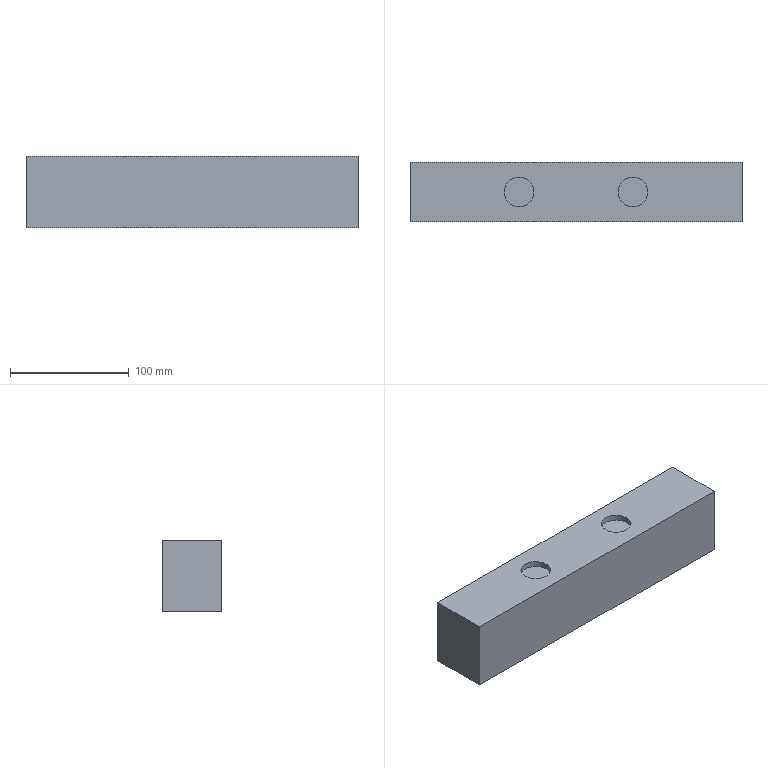Part | STEP file | 1 solid | 12 faces | box 280 x 50 x 60 mm | volume 835091 mm3 | plane 8 | cylinder 4 | commonest cylinder face diameters 25 x4
STEP:
#1=CARTESIAN_POINT('',(0.,0.,0.));
#2=DIRECTION('',(0.,0.,1.));
#3=DIRECTION('',(1.,0.,0.));
#4=AXIS2_PLACEMENT_3D('',#1,#2,#3);
#5=CARTESIAN_POINT('',(-60.5,0.,60.));
#6=VERTEX_POINT('',#5);
#7=CARTESIAN_POINT('',(-60.5,0.,55.));
#8=VERTEX_POINT('',#7);
#9=CARTESIAN_POINT('',(-60.5,0.,55.));
#10=DIRECTION('',(0.,0.,-1.));
#11=VECTOR('',#10,1.);
#12=LINE('',#9,#11);
#13=CARTESIAN_POINT('',(-48.,0.,55.));
#14=DIRECTION('',(0.,0.,-1.));
#15=DIRECTION('',(-1.,0.,0.));
#16=AXIS2_PLACEMENT_3D('',#13,#14,#15);
#17=CYLINDRICAL_SURFACE('',#16,12.5);
#18=CARTESIAN_POINT('',(6.283,0.));
#19=DIRECTION('',(0.,1.));
#20=VECTOR('',#19,1.);
#21=LINE('',#18,#20);
#22=(GEOMETRIC_REPRESENTATION_CONTEXT(2)PARAMETRIC_REPRESENTATION_CONTEXT()REPRESENTATION_CONTEXT('',''));
#23=DEFINITIONAL_REPRESENTATION('',(#21),#22);
#24=PCURVE('',#17,#23);
#25=CARTESIAN_POINT('',(-48.,0.,55.));
#26=DIRECTION('',(0.,0.,-1.));
#27=DIRECTION('',(-1.,0.,0.));
#28=AXIS2_PLACEMENT_3D('',#25,#26,#27);
#29=CYLINDRICAL_SURFACE('',#28,12.5);
#30=CARTESIAN_POINT('',(0.,0.));
#31=DIRECTION('',(0.,1.));
#32=VECTOR('',#31,1.);
#33=LINE('',#30,#32);
#34=(GEOMETRIC_REPRESENTATION_CONTEXT(2)PARAMETRIC_REPRESENTATION_CONTEXT()REPRESENTATION_CONTEXT('',''));
#35=DEFINITIONAL_REPRESENTATION('',(#33),#34);
#36=PCURVE('',#29,#35);
#37=SURFACE_CURVE('',#12,(#24,#36),.PCURVE_S1.);
#38=EDGE_CURVE('',#6,#8,#37,.T.);
#39=ORIENTED_EDGE('',*,*,#38,.T.);
#40=CARTESIAN_POINT('',(-35.5,0.,55.));
#41=VERTEX_POINT('',#40);
#42=CARTESIAN_POINT('',(-48.,0.,55.));
#43=DIRECTION('',(0.,0.,1.));
#44=DIRECTION('',(-1.,0.,0.));
#45=AXIS2_PLACEMENT_3D('',#42,#43,#44);
#46=CIRCLE('',#45,12.5);
#47=CARTESIAN_POINT('',(6.283,0.));
#48=DIRECTION('',(-1.,0.));
#49=VECTOR('',#48,1.);
#50=LINE('',#47,#49);
#51=(GEOMETRIC_REPRESENTATION_CONTEXT(2)PARAMETRIC_REPRESENTATION_CONTEXT()REPRESENTATION_CONTEXT('',''));
#52=DEFINITIONAL_REPRESENTATION('',(#50),#51);
#53=PCURVE('',#17,#52);
#54=CARTESIAN_POINT('',(-48.,0.,55.));
#55=DIRECTION('',(0.,0.,1.));
#56=DIRECTION('',(1.,0.,0.));
#57=AXIS2_PLACEMENT_3D('',#54,#55,#56);
#58=PLANE('',#57);
#59=CARTESIAN_POINT('',(0.,0.));
#60=DIRECTION('',(-1.,0.));
#61=AXIS2_PLACEMENT_2D('',#59,#60);
#62=CIRCLE('',#61,12.5);
#63=(GEOMETRIC_REPRESENTATION_CONTEXT(2)PARAMETRIC_REPRESENTATION_CONTEXT()REPRESENTATION_CONTEXT('',''));
#64=DEFINITIONAL_REPRESENTATION('',(#62),#63);
#65=PCURVE('',#58,#64);
#66=SURFACE_CURVE('',#46,(#53,#65),.PCURVE_S1.);
#67=EDGE_CURVE('',#8,#41,#66,.T.);
#68=ORIENTED_EDGE('',*,*,#67,.T.);
#69=CARTESIAN_POINT('',(-35.5,0.,60.));
#70=VERTEX_POINT('',#69);
#71=CARTESIAN_POINT('',(-35.5,0.,55.));
#72=DIRECTION('',(0.,0.,-1.));
#73=VECTOR('',#72,1.);
#74=LINE('',#71,#73);
#75=CARTESIAN_POINT('',(3.142,0.));
#76=DIRECTION('',(0.,1.));
#77=VECTOR('',#76,1.);
#78=LINE('',#75,#77);
#79=(GEOMETRIC_REPRESENTATION_CONTEXT(2)PARAMETRIC_REPRESENTATION_CONTEXT()REPRESENTATION_CONTEXT('',''));
#80=DEFINITIONAL_REPRESENTATION('',(#78),#79);
#81=PCURVE('',#17,#80);
#82=CARTESIAN_POINT('',(3.142,0.));
#83=DIRECTION('',(0.,1.));
#84=VECTOR('',#83,1.);
#85=LINE('',#82,#84);
#86=(GEOMETRIC_REPRESENTATION_CONTEXT(2)PARAMETRIC_REPRESENTATION_CONTEXT()REPRESENTATION_CONTEXT('',''));
#87=DEFINITIONAL_REPRESENTATION('',(#85),#86);
#88=PCURVE('',#29,#87);
#89=SURFACE_CURVE('',#74,(#81,#88),.PCURVE_S1.);
#90=EDGE_CURVE('',#70,#41,#89,.T.);
#91=ORIENTED_EDGE('',*,*,#90,.F.);
#92=CARTESIAN_POINT('',(-48.,0.,60.));
#93=DIRECTION('',(0.,0.,-1.));
#94=DIRECTION('',(-1.,0.,0.));
#95=AXIS2_PLACEMENT_3D('',#92,#93,#94);
#96=CIRCLE('',#95,12.5);
#97=CARTESIAN_POINT('',(0.,-5.));
#98=DIRECTION('',(1.,0.));
#99=VECTOR('',#98,1.);
#100=LINE('',#97,#99);
#101=(GEOMETRIC_REPRESENTATION_CONTEXT(2)PARAMETRIC_REPRESENTATION_CONTEXT()REPRESENTATION_CONTEXT('',''));
#102=DEFINITIONAL_REPRESENTATION('',(#100),#101);
#103=PCURVE('',#17,#102);
#104=CARTESIAN_POINT('',(0.,0.,60.));
#105=DIRECTION('',(0.,0.,1.));
#106=DIRECTION('',(1.,0.,0.));
#107=AXIS2_PLACEMENT_3D('',#104,#105,#106);
#108=PLANE('',#107);
#109=CARTESIAN_POINT('',(-60.5,0.));
#110=CARTESIAN_POINT('',(-60.5,21.651));
#111=CARTESIAN_POINT('',(-41.75,10.825));
#112=CARTESIAN_POINT('',(-23.,0.));
#113=CARTESIAN_POINT('',(-41.75,-10.825));
#114=CARTESIAN_POINT('',(-60.5,-21.651));
#115=CARTESIAN_POINT('',(-60.5,0.));
#116=(BOUNDED_CURVE()B_SPLINE_CURVE(2,(#109,#110,#111,#112,#113,#114,#115),.UNSPECIFIED.,.T.,.F.)B_SPLINE_CURVE_WITH_KNOTS((1,2,2,2,2,1),(-2.094,0.,2.094,4.189,6.283,8.378),.UNSPECIFIED.)CURVE()GEOMETRIC_REPRESENTATION_ITEM()RATIONAL_B_SPLINE_CURVE((1.,0.5,1.,0.5,1.,0.5,1.))REPRESENTATION_ITEM(''));
#117=(GEOMETRIC_REPRESENTATION_CONTEXT(2)PARAMETRIC_REPRESENTATION_CONTEXT()REPRESENTATION_CONTEXT('',''));
#118=DEFINITIONAL_REPRESENTATION('',(#116),#117);
#119=PCURVE('',#108,#118);
#120=SURFACE_CURVE('',#96,(#103,#119),.PCURVE_S1.);
#121=EDGE_CURVE('',#70,#6,#120,.T.);
#122=ORIENTED_EDGE('',*,*,#121,.T.);
#123=EDGE_LOOP('',(#39,#68,#91,#122));
#124=FACE_BOUND('',#123,.F.);
#125=ADVANCED_FACE('',(#124),#17,.F.);
#126=CARTESIAN_POINT('',(35.5,0.,60.));
#127=VERTEX_POINT('',#126);
#128=CARTESIAN_POINT('',(35.5,0.,55.));
#129=VERTEX_POINT('',#128);
#130=CARTESIAN_POINT('',(35.5,0.,55.));
#131=DIRECTION('',(0.,0.,-1.));
#132=VECTOR('',#131,1.);
#133=LINE('',#130,#132);
#134=CARTESIAN_POINT('',(48.,0.,55.));
#135=DIRECTION('',(0.,0.,-1.));
#136=DIRECTION('',(-1.,0.,0.));
#137=AXIS2_PLACEMENT_3D('',#134,#135,#136);
#138=CYLINDRICAL_SURFACE('',#137,12.5);
#139=CARTESIAN_POINT('',(6.283,0.));
#140=DIRECTION('',(0.,1.));
#141=VECTOR('',#140,1.);
#142=LINE('',#139,#141);
#143=(GEOMETRIC_REPRESENTATION_CONTEXT(2)PARAMETRIC_REPRESENTATION_CONTEXT()REPRESENTATION_CONTEXT('',''));
#144=DEFINITIONAL_REPRESENTATION('',(#142),#143);
#145=PCURVE('',#138,#144);
#146=CARTESIAN_POINT('',(48.,0.,55.));
#147=DIRECTION('',(0.,0.,-1.));
#148=DIRECTION('',(-1.,0.,0.));
#149=AXIS2_PLACEMENT_3D('',#146,#147,#148);
#150=CYLINDRICAL_SURFACE('',#149,12.5);
#151=CARTESIAN_POINT('',(0.,0.));
#152=DIRECTION('',(0.,1.));
#153=VECTOR('',#152,1.);
#154=LINE('',#151,#153);
#155=(GEOMETRIC_REPRESENTATION_CONTEXT(2)PARAMETRIC_REPRESENTATION_CONTEXT()REPRESENTATION_CONTEXT('',''));
#156=DEFINITIONAL_REPRESENTATION('',(#154),#155);
#157=PCURVE('',#150,#156);
#158=SURFACE_CURVE('',#133,(#145,#157),.PCURVE_S1.);
#159=EDGE_CURVE('',#127,#129,#158,.T.);
#160=ORIENTED_EDGE('',*,*,#159,.T.);
#161=CARTESIAN_POINT('',(60.5,0.,55.));
#162=VERTEX_POINT('',#161);
#163=CARTESIAN_POINT('',(48.,0.,55.));
#164=DIRECTION('',(0.,0.,1.));
#165=DIRECTION('',(-1.,0.,0.));
#166=AXIS2_PLACEMENT_3D('',#163,#164,#165);
#167=CIRCLE('',#166,12.5);
#168=CARTESIAN_POINT('',(6.283,0.));
#169=DIRECTION('',(-1.,0.));
#170=VECTOR('',#169,1.);
#171=LINE('',#168,#170);
#172=(GEOMETRIC_REPRESENTATION_CONTEXT(2)PARAMETRIC_REPRESENTATION_CONTEXT()REPRESENTATION_CONTEXT('',''));
#173=DEFINITIONAL_REPRESENTATION('',(#171),#172);
#174=PCURVE('',#138,#173);
#175=CARTESIAN_POINT('',(48.,0.,55.));
#176=DIRECTION('',(0.,0.,-1.));
#177=DIRECTION('',(-1.,0.,0.));
#178=AXIS2_PLACEMENT_3D('',#175,#176,#177);
#179=PLANE('',#178);
#180=CARTESIAN_POINT('',(12.5,0.));
#181=CARTESIAN_POINT('',(12.5,-21.651));
#182=CARTESIAN_POINT('',(-6.25,-10.825));
#183=CARTESIAN_POINT('',(-25.,0.));
#184=CARTESIAN_POINT('',(-6.25,10.825));
#185=CARTESIAN_POINT('',(12.5,21.651));
#186=CARTESIAN_POINT('',(12.5,0.));
#187=(BOUNDED_CURVE()B_SPLINE_CURVE(2,(#180,#181,#182,#183,#184,#185,#186),.UNSPECIFIED.,.T.,.F.)B_SPLINE_CURVE_WITH_KNOTS((1,2,2,2,2,1),(-2.094,0.,2.094,4.189,6.283,8.378),.UNSPECIFIED.)CURVE()GEOMETRIC_REPRESENTATION_ITEM()RATIONAL_B_SPLINE_CURVE((1.,0.5,1.,0.5,1.,0.5,1.))REPRESENTATION_ITEM(''));
#188=(GEOMETRIC_REPRESENTATION_CONTEXT(2)PARAMETRIC_REPRESENTATION_CONTEXT()REPRESENTATION_CONTEXT('',''));
#189=DEFINITIONAL_REPRESENTATION('',(#187),#188);
#190=PCURVE('',#179,#189);
#191=SURFACE_CURVE('',#167,(#174,#190),.PCURVE_S1.);
#192=EDGE_CURVE('',#129,#162,#191,.T.);
#193=ORIENTED_EDGE('',*,*,#192,.T.);
#194=CARTESIAN_POINT('',(60.5,0.,60.));
#195=VERTEX_POINT('',#194);
#196=CARTESIAN_POINT('',(60.5,0.,55.));
#197=DIRECTION('',(0.,0.,-1.));
#198=VECTOR('',#197,1.);
#199=LINE('',#196,#198);
#200=CARTESIAN_POINT('',(3.142,0.));
#201=DIRECTION('',(0.,1.));
#202=VECTOR('',#201,1.);
#203=LINE('',#200,#202);
#204=(GEOMETRIC_REPRESENTATION_CONTEXT(2)PARAMETRIC_REPRESENTATION_CONTEXT()REPRESENTATION_CONTEXT('',''));
#205=DEFINITIONAL_REPRESENTATION('',(#203),#204);
#206=PCURVE('',#138,#205);
#207=CARTESIAN_POINT('',(3.142,0.));
#208=DIRECTION('',(0.,1.));
#209=VECTOR('',#208,1.);
#210=LINE('',#207,#209);
#211=(GEOMETRIC_REPRESENTATION_CONTEXT(2)PARAMETRIC_REPRESENTATION_CONTEXT()REPRESENTATION_CONTEXT('',''));
#212=DEFINITIONAL_REPRESENTATION('',(#210),#211);
#213=PCURVE('',#150,#212);
#214=SURFACE_CURVE('',#199,(#206,#213),.PCURVE_S1.);
#215=EDGE_CURVE('',#195,#162,#214,.T.);
#216=ORIENTED_EDGE('',*,*,#215,.F.);
#217=CARTESIAN_POINT('',(48.,0.,60.));
#218=DIRECTION('',(0.,0.,-1.));
#219=DIRECTION('',(-1.,0.,0.));
#220=AXIS2_PLACEMENT_3D('',#217,#218,#219);
#221=CIRCLE('',#220,12.5);
#222=CARTESIAN_POINT('',(0.,-5.));
#223=DIRECTION('',(1.,0.));
#224=VECTOR('',#223,1.);
#225=LINE('',#222,#224);
#226=(GEOMETRIC_REPRESENTATION_CONTEXT(2)PARAMETRIC_REPRESENTATION_CONTEXT()REPRESENTATION_CONTEXT('',''));
#227=DEFINITIONAL_REPRESENTATION('',(#225),#226);
#228=PCURVE('',#138,#227);
#229=CARTESIAN_POINT('',(35.5,0.));
#230=CARTESIAN_POINT('',(35.5,21.651));
#231=CARTESIAN_POINT('',(54.25,10.825));
#232=CARTESIAN_POINT('',(73.,0.));
#233=CARTESIAN_POINT('',(54.25,-10.825));
#234=CARTESIAN_POINT('',(35.5,-21.651));
#235=CARTESIAN_POINT('',(35.5,0.));
#236=(BOUNDED_CURVE()B_SPLINE_CURVE(2,(#229,#230,#231,#232,#233,#234,#235),.UNSPECIFIED.,.T.,.F.)B_SPLINE_CURVE_WITH_KNOTS((1,2,2,2,2,1),(-2.094,0.,2.094,4.189,6.283,8.378),.UNSPECIFIED.)CURVE()GEOMETRIC_REPRESENTATION_ITEM()RATIONAL_B_SPLINE_CURVE((1.,0.5,1.,0.5,1.,0.5,1.))REPRESENTATION_ITEM(''));
#237=(GEOMETRIC_REPRESENTATION_CONTEXT(2)PARAMETRIC_REPRESENTATION_CONTEXT()REPRESENTATION_CONTEXT('',''));
#238=DEFINITIONAL_REPRESENTATION('',(#236),#237);
#239=PCURVE('',#108,#238);
#240=SURFACE_CURVE('',#221,(#228,#239),.PCURVE_S1.);
#241=EDGE_CURVE('',#195,#127,#240,.T.);
#242=ORIENTED_EDGE('',*,*,#241,.T.);
#243=EDGE_LOOP('',(#160,#193,#216,#242));
#244=FACE_BOUND('',#243,.F.);
#245=ADVANCED_FACE('',(#244),#138,.F.);
#246=CARTESIAN_POINT('',(-140.,25.,60.));
#247=VERTEX_POINT('',#246);
#248=CARTESIAN_POINT('',(-140.,25.,0.));
#249=VERTEX_POINT('',#248);
#250=CARTESIAN_POINT('',(-140.,25.,60.));
#251=DIRECTION('',(0.,0.,-1.));
#252=VECTOR('',#251,1.);
#253=LINE('',#250,#252);
#254=CARTESIAN_POINT('',(-140.,25.,60.));
#255=DIRECTION('',(0.,-1.,0.));
#256=DIRECTION('',(0.,0.,-1.));
#257=AXIS2_PLACEMENT_3D('',#254,#255,#256);
#258=PLANE('',#257);
#259=CARTESIAN_POINT('',(0.,0.));
#260=DIRECTION('',(1.,0.));
#261=VECTOR('',#260,1.);
#262=LINE('',#259,#261);
#263=(GEOMETRIC_REPRESENTATION_CONTEXT(2)PARAMETRIC_REPRESENTATION_CONTEXT()REPRESENTATION_CONTEXT('',''));
#264=DEFINITIONAL_REPRESENTATION('',(#262),#263);
#265=PCURVE('',#258,#264);
#266=CARTESIAN_POINT('',(-140.,25.,60.));
#267=DIRECTION('',(1.,0.,0.));
#268=DIRECTION('',(0.,0.,-1.));
#269=AXIS2_PLACEMENT_3D('',#266,#267,#268);
#270=PLANE('',#269);
#271=CARTESIAN_POINT('',(0.,0.));
#272=DIRECTION('',(1.,0.));
#273=VECTOR('',#272,1.);
#274=LINE('',#271,#273);
#275=(GEOMETRIC_REPRESENTATION_CONTEXT(2)PARAMETRIC_REPRESENTATION_CONTEXT()REPRESENTATION_CONTEXT('',''));
#276=DEFINITIONAL_REPRESENTATION('',(#274),#275);
#277=PCURVE('',#270,#276);
#278=SURFACE_CURVE('',#253,(#265,#277),.PCURVE_S1.);
#279=EDGE_CURVE('',#247,#249,#278,.T.);
#280=ORIENTED_EDGE('',*,*,#279,.F.);
#281=CARTESIAN_POINT('',(140.,25.,60.));
#282=VERTEX_POINT('',#281);
#283=CARTESIAN_POINT('',(-140.,25.,60.));
#284=DIRECTION('',(-1.,0.,0.));
#285=VECTOR('',#284,1.);
#286=LINE('',#283,#285);
#287=CARTESIAN_POINT('',(0.,0.));
#288=DIRECTION('',(0.,-1.));
#289=VECTOR('',#288,1.);
#290=LINE('',#287,#289);
#291=(GEOMETRIC_REPRESENTATION_CONTEXT(2)PARAMETRIC_REPRESENTATION_CONTEXT()REPRESENTATION_CONTEXT('',''));
#292=DEFINITIONAL_REPRESENTATION('',(#290),#291);
#293=PCURVE('',#258,#292);
#294=CARTESIAN_POINT('',(-140.,25.));
#295=DIRECTION('',(-1.,0.));
#296=VECTOR('',#295,1.);
#297=LINE('',#294,#296);
#298=(GEOMETRIC_REPRESENTATION_CONTEXT(2)PARAMETRIC_REPRESENTATION_CONTEXT()REPRESENTATION_CONTEXT('',''));
#299=DEFINITIONAL_REPRESENTATION('',(#297),#298);
#300=PCURVE('',#108,#299);
#301=SURFACE_CURVE('',#286,(#293,#300),.PCURVE_S1.);
#302=EDGE_CURVE('',#282,#247,#301,.T.);
#303=ORIENTED_EDGE('',*,*,#302,.F.);
#304=CARTESIAN_POINT('',(140.,25.,0.));
#305=VERTEX_POINT('',#304);
#306=CARTESIAN_POINT('',(140.,25.,60.));
#307=DIRECTION('',(0.,0.,1.));
#308=VECTOR('',#307,1.);
#309=LINE('',#306,#308);
#310=CARTESIAN_POINT('',(0.,280.));
#311=DIRECTION('',(-1.,0.));
#312=VECTOR('',#311,1.);
#313=LINE('',#310,#312);
#314=(GEOMETRIC_REPRESENTATION_CONTEXT(2)PARAMETRIC_REPRESENTATION_CONTEXT()REPRESENTATION_CONTEXT('',''));
#315=DEFINITIONAL_REPRESENTATION('',(#313),#314);
#316=PCURVE('',#258,#315);
#317=CARTESIAN_POINT('',(140.,25.,60.));
#318=DIRECTION('',(-1.,0.,0.));
#319=DIRECTION('',(0.,0.,1.));
#320=AXIS2_PLACEMENT_3D('',#317,#318,#319);
#321=PLANE('',#320);
#322=CARTESIAN_POINT('',(0.,0.));
#323=DIRECTION('',(1.,0.));
#324=VECTOR('',#323,1.);
#325=LINE('',#322,#324);
#326=(GEOMETRIC_REPRESENTATION_CONTEXT(2)PARAMETRIC_REPRESENTATION_CONTEXT()REPRESENTATION_CONTEXT('',''));
#327=DEFINITIONAL_REPRESENTATION('',(#325),#326);
#328=PCURVE('',#321,#327);
#329=SURFACE_CURVE('',#309,(#316,#328),.PCURVE_S1.);
#330=EDGE_CURVE('',#305,#282,#329,.T.);
#331=ORIENTED_EDGE('',*,*,#330,.F.);
#332=CARTESIAN_POINT('',(-140.,25.,0.));
#333=DIRECTION('',(1.,0.,0.));
#334=VECTOR('',#333,1.);
#335=LINE('',#332,#334);
#336=CARTESIAN_POINT('',(60.,0.));
#337=DIRECTION('',(0.,1.));
#338=VECTOR('',#337,1.);
#339=LINE('',#336,#338);
#340=(GEOMETRIC_REPRESENTATION_CONTEXT(2)PARAMETRIC_REPRESENTATION_CONTEXT()REPRESENTATION_CONTEXT('',''));
#341=DEFINITIONAL_REPRESENTATION('',(#339),#340);
#342=PCURVE('',#258,#341);
#343=CARTESIAN_POINT('',(0.,0.,0.));
#344=DIRECTION('',(0.,0.,1.));
#345=DIRECTION('',(1.,0.,0.));
#346=AXIS2_PLACEMENT_3D('',#343,#344,#345);
#347=PLANE('',#346);
#348=CARTESIAN_POINT('',(-140.,25.));
#349=DIRECTION('',(1.,0.));
#350=VECTOR('',#349,1.);
#351=LINE('',#348,#350);
#352=(GEOMETRIC_REPRESENTATION_CONTEXT(2)PARAMETRIC_REPRESENTATION_CONTEXT()REPRESENTATION_CONTEXT('',''));
#353=DEFINITIONAL_REPRESENTATION('',(#351),#352);
#354=PCURVE('',#347,#353);
#355=SURFACE_CURVE('',#335,(#342,#354),.PCURVE_S1.);
#356=EDGE_CURVE('',#249,#305,#355,.T.);
#357=ORIENTED_EDGE('',*,*,#356,.F.);
#358=EDGE_LOOP('',(#280,#303,#331,#357));
#359=FACE_BOUND('',#358,.T.);
#360=ADVANCED_FACE('',(#359),#258,.F.);
#361=CARTESIAN_POINT('',(-140.,-25.,0.));
#362=VERTEX_POINT('',#361);
#363=CARTESIAN_POINT('',(140.,-25.,0.));
#364=VERTEX_POINT('',#363);
#365=CARTESIAN_POINT('',(0.,-25.,0.));
#366=DIRECTION('',(1.,0.,0.));
#367=VECTOR('',#366,1.);
#368=LINE('',#365,#367);
#369=CARTESIAN_POINT('',(0.,-25.));
#370=DIRECTION('',(1.,0.));
#371=VECTOR('',#370,1.);
#372=LINE('',#369,#371);
#373=(GEOMETRIC_REPRESENTATION_CONTEXT(2)PARAMETRIC_REPRESENTATION_CONTEXT()REPRESENTATION_CONTEXT('',''));
#374=DEFINITIONAL_REPRESENTATION('',(#372),#373);
#375=PCURVE('',#347,#374);
#376=CARTESIAN_POINT('',(-140.,-25.,60.));
#377=DIRECTION('',(0.,1.,0.));
#378=DIRECTION('',(0.,0.,1.));
#379=AXIS2_PLACEMENT_3D('',#376,#377,#378);
#380=PLANE('',#379);
#381=CARTESIAN_POINT('',(-60.,140.));
#382=DIRECTION('',(0.,1.));
#383=VECTOR('',#382,1.);
#384=LINE('',#381,#383);
#385=(GEOMETRIC_REPRESENTATION_CONTEXT(2)PARAMETRIC_REPRESENTATION_CONTEXT()REPRESENTATION_CONTEXT('',''));
#386=DEFINITIONAL_REPRESENTATION('',(#384),#385);
#387=PCURVE('',#380,#386);
#388=SURFACE_CURVE('',#368,(#375,#387),.PCURVE_S1.);
#389=EDGE_CURVE('',#362,#364,#388,.T.);
#390=ORIENTED_EDGE('',*,*,#389,.F.);
#391=CARTESIAN_POINT('',(-140.,0.,0.));
#392=DIRECTION('',(0.,-1.,0.));
#393=VECTOR('',#392,1.);
#394=LINE('',#391,#393);
#395=CARTESIAN_POINT('',(-140.,0.));
#396=DIRECTION('',(0.,-1.));
#397=VECTOR('',#396,1.);
#398=LINE('',#395,#397);
#399=(GEOMETRIC_REPRESENTATION_CONTEXT(2)PARAMETRIC_REPRESENTATION_CONTEXT()REPRESENTATION_CONTEXT('',''));
#400=DEFINITIONAL_REPRESENTATION('',(#398),#399);
#401=PCURVE('',#347,#400);
#402=CARTESIAN_POINT('',(60.,-25.));
#403=DIRECTION('',(0.,-1.));
#404=VECTOR('',#403,1.);
#405=LINE('',#402,#404);
#406=(GEOMETRIC_REPRESENTATION_CONTEXT(2)PARAMETRIC_REPRESENTATION_CONTEXT()REPRESENTATION_CONTEXT('',''));
#407=DEFINITIONAL_REPRESENTATION('',(#405),#406);
#408=PCURVE('',#270,#407);
#409=SURFACE_CURVE('',#394,(#401,#408),.PCURVE_S1.);
#410=EDGE_CURVE('',#249,#362,#409,.T.);
#411=ORIENTED_EDGE('',*,*,#410,.F.);
#412=ORIENTED_EDGE('',*,*,#356,.T.);
#413=CARTESIAN_POINT('',(140.,0.,0.));
#414=DIRECTION('',(0.,1.,0.));
#415=VECTOR('',#414,1.);
#416=LINE('',#413,#415);
#417=CARTESIAN_POINT('',(140.,0.));
#418=DIRECTION('',(0.,1.));
#419=VECTOR('',#418,1.);
#420=LINE('',#417,#419);
#421=(GEOMETRIC_REPRESENTATION_CONTEXT(2)PARAMETRIC_REPRESENTATION_CONTEXT()REPRESENTATION_CONTEXT('',''));
#422=DEFINITIONAL_REPRESENTATION('',(#420),#421);
#423=PCURVE('',#347,#422);
#424=CARTESIAN_POINT('',(-60.,-25.));
#425=DIRECTION('',(0.,1.));
#426=VECTOR('',#425,1.);
#427=LINE('',#424,#426);
#428=(GEOMETRIC_REPRESENTATION_CONTEXT(2)PARAMETRIC_REPRESENTATION_CONTEXT()REPRESENTATION_CONTEXT('',''));
#429=DEFINITIONAL_REPRESENTATION('',(#427),#428);
#430=PCURVE('',#321,#429);
#431=SURFACE_CURVE('',#416,(#423,#430),.PCURVE_S1.);
#432=EDGE_CURVE('',#364,#305,#431,.T.);
#433=ORIENTED_EDGE('',*,*,#432,.F.);
#434=EDGE_LOOP('',(#390,#411,#412,#433));
#435=FACE_BOUND('',#434,.T.);
#436=ADVANCED_FACE('',(#435),#347,.F.);
#437=CARTESIAN_POINT('',(-140.,-25.,60.));
#438=VERTEX_POINT('',#437);
#439=CARTESIAN_POINT('',(-140.,-25.,60.));
#440=DIRECTION('',(0.,0.,-1.));
#441=VECTOR('',#440,1.);
#442=LINE('',#439,#441);
#443=CARTESIAN_POINT('',(0.,-50.));
#444=DIRECTION('',(1.,0.));
#445=VECTOR('',#444,1.);
#446=LINE('',#443,#445);
#447=(GEOMETRIC_REPRESENTATION_CONTEXT(2)PARAMETRIC_REPRESENTATION_CONTEXT()REPRESENTATION_CONTEXT('',''));
#448=DEFINITIONAL_REPRESENTATION('',(#446),#447);
#449=PCURVE('',#270,#448);
#450=CARTESIAN_POINT('',(0.,0.));
#451=DIRECTION('',(-1.,0.));
#452=VECTOR('',#451,1.);
#453=LINE('',#450,#452);
#454=(GEOMETRIC_REPRESENTATION_CONTEXT(2)PARAMETRIC_REPRESENTATION_CONTEXT()REPRESENTATION_CONTEXT('',''));
#455=DEFINITIONAL_REPRESENTATION('',(#453),#454);
#456=PCURVE('',#380,#455);
#457=SURFACE_CURVE('',#442,(#449,#456),.PCURVE_S1.);
#458=EDGE_CURVE('',#438,#362,#457,.T.);
#459=ORIENTED_EDGE('',*,*,#458,.F.);
#460=CARTESIAN_POINT('',(-140.,25.,60.));
#461=DIRECTION('',(0.,-1.,0.));
#462=VECTOR('',#461,1.);
#463=LINE('',#460,#462);
#464=CARTESIAN_POINT('',(0.,0.));
#465=DIRECTION('',(0.,-1.));
#466=VECTOR('',#465,1.);
#467=LINE('',#464,#466);
#468=(GEOMETRIC_REPRESENTATION_CONTEXT(2)PARAMETRIC_REPRESENTATION_CONTEXT()REPRESENTATION_CONTEXT('',''));
#469=DEFINITIONAL_REPRESENTATION('',(#467),#468);
#470=PCURVE('',#270,#469);
#471=CARTESIAN_POINT('',(-140.,25.));
#472=DIRECTION('',(0.,-1.));
#473=VECTOR('',#472,1.);
#474=LINE('',#471,#473);
#475=(GEOMETRIC_REPRESENTATION_CONTEXT(2)PARAMETRIC_REPRESENTATION_CONTEXT()REPRESENTATION_CONTEXT('',''));
#476=DEFINITIONAL_REPRESENTATION('',(#474),#475);
#477=PCURVE('',#108,#476);
#478=SURFACE_CURVE('',#463,(#470,#477),.PCURVE_S1.);
#479=EDGE_CURVE('',#247,#438,#478,.T.);
#480=ORIENTED_EDGE('',*,*,#479,.F.);
#481=ORIENTED_EDGE('',*,*,#279,.T.);
#482=ORIENTED_EDGE('',*,*,#410,.T.);
#483=EDGE_LOOP('',(#459,#480,#481,#482));
#484=FACE_BOUND('',#483,.T.);
#485=ADVANCED_FACE('',(#484),#270,.F.);
#486=CARTESIAN_POINT('',(-48.,0.,60.));
#487=DIRECTION('',(0.,0.,-1.));
#488=DIRECTION('',(-1.,0.,0.));
#489=AXIS2_PLACEMENT_3D('',#486,#487,#488);
#490=CIRCLE('',#489,12.5);
#491=CARTESIAN_POINT('',(-60.5,0.));
#492=CARTESIAN_POINT('',(-60.5,21.651));
#493=CARTESIAN_POINT('',(-41.75,10.825));
#494=CARTESIAN_POINT('',(-23.,0.));
#495=CARTESIAN_POINT('',(-41.75,-10.825));
#496=CARTESIAN_POINT('',(-60.5,-21.651));
#497=CARTESIAN_POINT('',(-60.5,0.));
#498=(BOUNDED_CURVE()B_SPLINE_CURVE(2,(#491,#492,#493,#494,#495,#496,#497),.UNSPECIFIED.,.T.,.F.)B_SPLINE_CURVE_WITH_KNOTS((1,2,2,2,2,1),(-2.094,0.,2.094,4.189,6.283,8.378),.UNSPECIFIED.)CURVE()GEOMETRIC_REPRESENTATION_ITEM()RATIONAL_B_SPLINE_CURVE((1.,0.5,1.,0.5,1.,0.5,1.))REPRESENTATION_ITEM(''));
#499=(GEOMETRIC_REPRESENTATION_CONTEXT(2)PARAMETRIC_REPRESENTATION_CONTEXT()REPRESENTATION_CONTEXT('',''));
#500=DEFINITIONAL_REPRESENTATION('',(#498),#499);
#501=PCURVE('',#108,#500);
#502=CARTESIAN_POINT('',(0.,-5.));
#503=DIRECTION('',(1.,0.));
#504=VECTOR('',#503,1.);
#505=LINE('',#502,#504);
#506=(GEOMETRIC_REPRESENTATION_CONTEXT(2)PARAMETRIC_REPRESENTATION_CONTEXT()REPRESENTATION_CONTEXT('',''));
#507=DEFINITIONAL_REPRESENTATION('',(#505),#506);
#508=PCURVE('',#29,#507);
#509=SURFACE_CURVE('',#490,(#501,#508),.PCURVE_S1.);
#510=EDGE_CURVE('',#6,#70,#509,.T.);
#511=ORIENTED_EDGE('',*,*,#510,.T.);
#512=ORIENTED_EDGE('',*,*,#121,.T.);
#513=EDGE_LOOP('',(#511,#512));
#514=FACE_BOUND('',#513,.T.);
#515=CARTESIAN_POINT('',(48.,0.,60.));
#516=DIRECTION('',(0.,0.,-1.));
#517=DIRECTION('',(-1.,0.,0.));
#518=AXIS2_PLACEMENT_3D('',#515,#516,#517);
#519=CIRCLE('',#518,12.5);
#520=CARTESIAN_POINT('',(35.5,0.));
#521=CARTESIAN_POINT('',(35.5,21.651));
#522=CARTESIAN_POINT('',(54.25,10.825));
#523=CARTESIAN_POINT('',(73.,0.));
#524=CARTESIAN_POINT('',(54.25,-10.825));
#525=CARTESIAN_POINT('',(35.5,-21.651));
#526=CARTESIAN_POINT('',(35.5,0.));
#527=(BOUNDED_CURVE()B_SPLINE_CURVE(2,(#520,#521,#522,#523,#524,#525,#526),.UNSPECIFIED.,.T.,.F.)B_SPLINE_CURVE_WITH_KNOTS((1,2,2,2,2,1),(-2.094,0.,2.094,4.189,6.283,8.378),.UNSPECIFIED.)CURVE()GEOMETRIC_REPRESENTATION_ITEM()RATIONAL_B_SPLINE_CURVE((1.,0.5,1.,0.5,1.,0.5,1.))REPRESENTATION_ITEM(''));
#528=(GEOMETRIC_REPRESENTATION_CONTEXT(2)PARAMETRIC_REPRESENTATION_CONTEXT()REPRESENTATION_CONTEXT('',''));
#529=DEFINITIONAL_REPRESENTATION('',(#527),#528);
#530=PCURVE('',#108,#529);
#531=CARTESIAN_POINT('',(0.,-5.));
#532=DIRECTION('',(1.,0.));
#533=VECTOR('',#532,1.);
#534=LINE('',#531,#533);
#535=(GEOMETRIC_REPRESENTATION_CONTEXT(2)PARAMETRIC_REPRESENTATION_CONTEXT()REPRESENTATION_CONTEXT('',''));
#536=DEFINITIONAL_REPRESENTATION('',(#534),#535);
#537=PCURVE('',#150,#536);
#538=SURFACE_CURVE('',#519,(#530,#537),.PCURVE_S1.);
#539=EDGE_CURVE('',#127,#195,#538,.T.);
#540=ORIENTED_EDGE('',*,*,#539,.T.);
#541=ORIENTED_EDGE('',*,*,#241,.T.);
#542=EDGE_LOOP('',(#540,#541));
#543=FACE_BOUND('',#542,.T.);
#544=ORIENTED_EDGE('',*,*,#479,.T.);
#545=CARTESIAN_POINT('',(140.,-25.,60.));
#546=VERTEX_POINT('',#545);
#547=CARTESIAN_POINT('',(0.,-25.,60.));
#548=DIRECTION('',(1.,0.,0.));
#549=VECTOR('',#548,1.);
#550=LINE('',#547,#549);
#551=CARTESIAN_POINT('',(0.,-25.));
#552=DIRECTION('',(1.,0.));
#553=VECTOR('',#552,1.);
#554=LINE('',#551,#553);
#555=(GEOMETRIC_REPRESENTATION_CONTEXT(2)PARAMETRIC_REPRESENTATION_CONTEXT()REPRESENTATION_CONTEXT('',''));
#556=DEFINITIONAL_REPRESENTATION('',(#554),#555);
#557=PCURVE('',#108,#556);
#558=CARTESIAN_POINT('',(0.,140.));
#559=DIRECTION('',(0.,1.));
#560=VECTOR('',#559,1.);
#561=LINE('',#558,#560);
#562=(GEOMETRIC_REPRESENTATION_CONTEXT(2)PARAMETRIC_REPRESENTATION_CONTEXT()REPRESENTATION_CONTEXT('',''));
#563=DEFINITIONAL_REPRESENTATION('',(#561),#562);
#564=PCURVE('',#380,#563);
#565=SURFACE_CURVE('',#550,(#557,#564),.PCURVE_S1.);
#566=EDGE_CURVE('',#438,#546,#565,.T.);
#567=ORIENTED_EDGE('',*,*,#566,.T.);
#568=CARTESIAN_POINT('',(140.,0.,60.));
#569=DIRECTION('',(0.,1.,0.));
#570=VECTOR('',#569,1.);
#571=LINE('',#568,#570);
#572=CARTESIAN_POINT('',(140.,0.));
#573=DIRECTION('',(0.,1.));
#574=VECTOR('',#573,1.);
#575=LINE('',#572,#574);
#576=(GEOMETRIC_REPRESENTATION_CONTEXT(2)PARAMETRIC_REPRESENTATION_CONTEXT()REPRESENTATION_CONTEXT('',''));
#577=DEFINITIONAL_REPRESENTATION('',(#575),#576);
#578=PCURVE('',#108,#577);
#579=CARTESIAN_POINT('',(0.,-25.));
#580=DIRECTION('',(0.,1.));
#581=VECTOR('',#580,1.);
#582=LINE('',#579,#581);
#583=(GEOMETRIC_REPRESENTATION_CONTEXT(2)PARAMETRIC_REPRESENTATION_CONTEXT()REPRESENTATION_CONTEXT('',''));
#584=DEFINITIONAL_REPRESENTATION('',(#582),#583);
#585=PCURVE('',#321,#584);
#586=SURFACE_CURVE('',#571,(#578,#585),.PCURVE_S1.);
#587=EDGE_CURVE('',#546,#282,#586,.T.);
#588=ORIENTED_EDGE('',*,*,#587,.T.);
#589=ORIENTED_EDGE('',*,*,#302,.T.);
#590=EDGE_LOOP('',(#544,#567,#588,#589));
#591=FACE_BOUND('',#590,.T.);
#592=ADVANCED_FACE('',(#514,#543,#591),#108,.T.);
#593=ORIENTED_EDGE('',*,*,#330,.T.);
#594=ORIENTED_EDGE('',*,*,#587,.F.);
#595=CARTESIAN_POINT('',(140.,-25.,60.));
#596=DIRECTION('',(0.,0.,1.));
#597=VECTOR('',#596,1.);
#598=LINE('',#595,#597);
#599=CARTESIAN_POINT('',(0.,-50.));
#600=DIRECTION('',(1.,0.));
#601=VECTOR('',#600,1.);
#602=LINE('',#599,#601);
#603=(GEOMETRIC_REPRESENTATION_CONTEXT(2)PARAMETRIC_REPRESENTATION_CONTEXT()REPRESENTATION_CONTEXT('',''));
#604=DEFINITIONAL_REPRESENTATION('',(#602),#603);
#605=PCURVE('',#321,#604);
#606=CARTESIAN_POINT('',(0.,280.));
#607=DIRECTION('',(1.,0.));
#608=VECTOR('',#607,1.);
#609=LINE('',#606,#608);
#610=(GEOMETRIC_REPRESENTATION_CONTEXT(2)PARAMETRIC_REPRESENTATION_CONTEXT()REPRESENTATION_CONTEXT('',''));
#611=DEFINITIONAL_REPRESENTATION('',(#609),#610);
#612=PCURVE('',#380,#611);
#613=SURFACE_CURVE('',#598,(#605,#612),.PCURVE_S1.);
#614=EDGE_CURVE('',#364,#546,#613,.T.);
#615=ORIENTED_EDGE('',*,*,#614,.F.);
#616=ORIENTED_EDGE('',*,*,#432,.T.);
#617=EDGE_LOOP('',(#593,#594,#615,#616));
#618=FACE_BOUND('',#617,.T.);
#619=ADVANCED_FACE('',(#618),#321,.F.);
#620=ORIENTED_EDGE('',*,*,#614,.T.);
#621=ORIENTED_EDGE('',*,*,#566,.F.);
#622=ORIENTED_EDGE('',*,*,#458,.T.);
#623=ORIENTED_EDGE('',*,*,#389,.T.);
#624=EDGE_LOOP('',(#620,#621,#622,#623));
#625=FACE_BOUND('',#624,.T.);
#626=ADVANCED_FACE('',(#625),#380,.F.);
#627=CARTESIAN_POINT('',(-48.,0.,55.));
#628=DIRECTION('',(0.,0.,1.));
#629=DIRECTION('',(-1.,0.,0.));
#630=AXIS2_PLACEMENT_3D('',#627,#628,#629);
#631=CIRCLE('',#630,12.5);
#632=CARTESIAN_POINT('',(6.283,0.));
#633=DIRECTION('',(-1.,0.));
#634=VECTOR('',#633,1.);
#635=LINE('',#632,#634);
#636=(GEOMETRIC_REPRESENTATION_CONTEXT(2)PARAMETRIC_REPRESENTATION_CONTEXT()REPRESENTATION_CONTEXT('',''));
#637=DEFINITIONAL_REPRESENTATION('',(#635),#636);
#638=PCURVE('',#29,#637);
#639=CARTESIAN_POINT('',(0.,0.));
#640=DIRECTION('',(-1.,0.));
#641=AXIS2_PLACEMENT_2D('',#639,#640);
#642=CIRCLE('',#641,12.5);
#643=(GEOMETRIC_REPRESENTATION_CONTEXT(2)PARAMETRIC_REPRESENTATION_CONTEXT()REPRESENTATION_CONTEXT('',''));
#644=DEFINITIONAL_REPRESENTATION('',(#642),#643);
#645=PCURVE('',#58,#644);
#646=SURFACE_CURVE('',#631,(#638,#645),.PCURVE_S1.);
#647=EDGE_CURVE('',#41,#8,#646,.T.);
#648=ORIENTED_EDGE('',*,*,#647,.T.);
#649=ORIENTED_EDGE('',*,*,#38,.F.);
#650=ORIENTED_EDGE('',*,*,#510,.T.);
#651=ORIENTED_EDGE('',*,*,#90,.T.);
#652=EDGE_LOOP('',(#648,#649,#650,#651));
#653=FACE_BOUND('',#652,.F.);
#654=ADVANCED_FACE('',(#653),#29,.F.);
#655=CARTESIAN_POINT('',(48.,0.,55.));
#656=DIRECTION('',(0.,0.,1.));
#657=DIRECTION('',(-1.,0.,0.));
#658=AXIS2_PLACEMENT_3D('',#655,#656,#657);
#659=CIRCLE('',#658,12.5);
#660=CARTESIAN_POINT('',(6.283,0.));
#661=DIRECTION('',(-1.,0.));
#662=VECTOR('',#661,1.);
#663=LINE('',#660,#662);
#664=(GEOMETRIC_REPRESENTATION_CONTEXT(2)PARAMETRIC_REPRESENTATION_CONTEXT()REPRESENTATION_CONTEXT('',''));
#665=DEFINITIONAL_REPRESENTATION('',(#663),#664);
#666=PCURVE('',#150,#665);
#667=CARTESIAN_POINT('',(12.5,0.));
#668=CARTESIAN_POINT('',(12.5,-21.651));
#669=CARTESIAN_POINT('',(-6.25,-10.825));
#670=CARTESIAN_POINT('',(-25.,0.));
#671=CARTESIAN_POINT('',(-6.25,10.825));
#672=CARTESIAN_POINT('',(12.5,21.651));
#673=CARTESIAN_POINT('',(12.5,0.));
#674=(BOUNDED_CURVE()B_SPLINE_CURVE(2,(#667,#668,#669,#670,#671,#672,#673),.UNSPECIFIED.,.T.,.F.)B_SPLINE_CURVE_WITH_KNOTS((1,2,2,2,2,1),(-2.094,0.,2.094,4.189,6.283,8.378),.UNSPECIFIED.)CURVE()GEOMETRIC_REPRESENTATION_ITEM()RATIONAL_B_SPLINE_CURVE((1.,0.5,1.,0.5,1.,0.5,1.))REPRESENTATION_ITEM(''));
#675=(GEOMETRIC_REPRESENTATION_CONTEXT(2)PARAMETRIC_REPRESENTATION_CONTEXT()REPRESENTATION_CONTEXT('',''));
#676=DEFINITIONAL_REPRESENTATION('',(#674),#675);
#677=PCURVE('',#179,#676);
#678=SURFACE_CURVE('',#659,(#666,#677),.PCURVE_S1.);
#679=EDGE_CURVE('',#162,#129,#678,.T.);
#680=ORIENTED_EDGE('',*,*,#679,.T.);
#681=ORIENTED_EDGE('',*,*,#159,.F.);
#682=ORIENTED_EDGE('',*,*,#539,.T.);
#683=ORIENTED_EDGE('',*,*,#215,.T.);
#684=EDGE_LOOP('',(#680,#681,#682,#683));
#685=FACE_BOUND('',#684,.F.);
#686=ADVANCED_FACE('',(#685),#150,.F.);
#687=ORIENTED_EDGE('',*,*,#67,.T.);
#688=ORIENTED_EDGE('',*,*,#647,.T.);
#689=EDGE_LOOP('',(#687,#688));
#690=FACE_BOUND('',#689,.T.);
#691=ADVANCED_FACE('',(#690),#58,.T.);
#692=ORIENTED_EDGE('',*,*,#192,.T.);
#693=ORIENTED_EDGE('',*,*,#679,.T.);
#694=EDGE_LOOP('',(#692,#693));
#695=FACE_BOUND('',#694,.T.);
#696=ADVANCED_FACE('',(#695),#179,.F.);
#697=CLOSED_SHELL('',(#125,#245,#360,#436,#485,#592,#619,#626,#654,#686,#691,#696));
#698=MANIFOLD_SOLID_BREP('',#697);
#699=(LENGTH_UNIT()NAMED_UNIT(*)SI_UNIT(.MILLI.,.METRE.));
#700=UNCERTAINTY_MEASURE_WITH_UNIT(LENGTH_MEASURE(0.0000001),#699,'','');
#701=(NAMED_UNIT(*)PLANE_ANGLE_UNIT()SI_UNIT($,.RADIAN.));
#702=(NAMED_UNIT(*)SI_UNIT($,.STERADIAN.)SOLID_ANGLE_UNIT());
#703=(GEOMETRIC_REPRESENTATION_CONTEXT(3)GLOBAL_UNCERTAINTY_ASSIGNED_CONTEXT((#700))GLOBAL_UNIT_ASSIGNED_CONTEXT((#699,#701,#702))REPRESENTATION_CONTEXT('',''));
#704=ADVANCED_BREP_SHAPE_REPRESENTATION('',(#4,#698),#703);